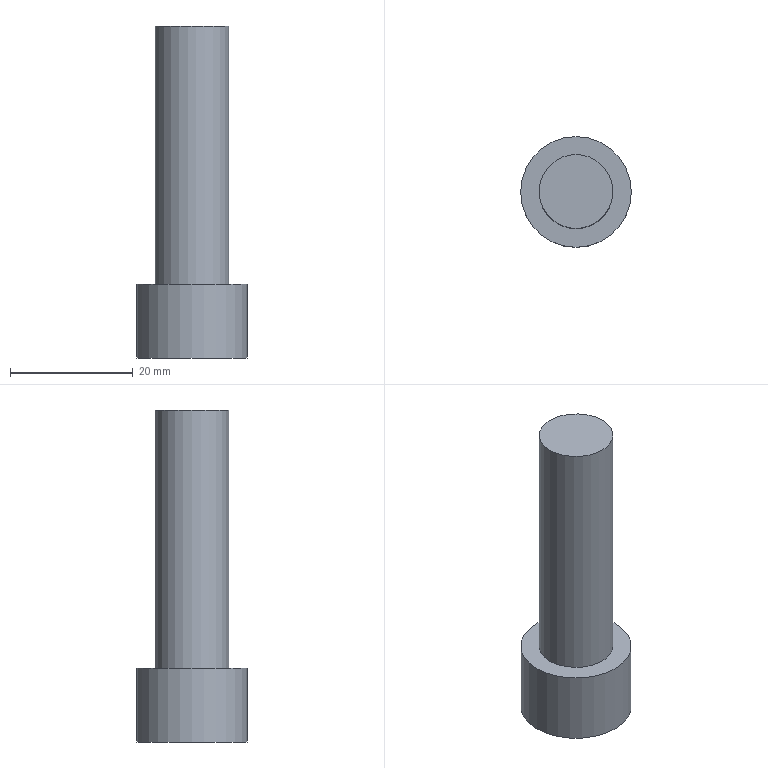Part | STEP file | solid 23 | 1 solid | 12 faces | box 18 x 18 x 54 mm | volume 7284 mm3 | plane 10 | cylinder 2 | commonest cylinder face diameters 12 x1 18 x1